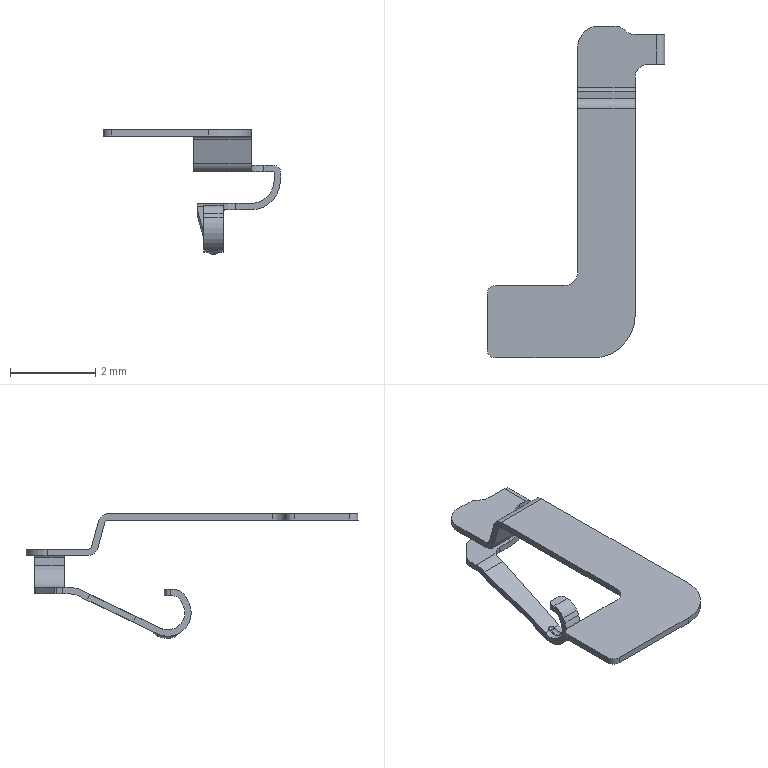Part | STEP file | p9-frame-02 | 1 solid | 70 faces | box 4.174 x 7.792 x 2.928 mm | volume 2.811 mm3 | plane 31 | cylinder 29 | spline 10 | commonest cylinder face diameters 0.4 x5 0.6 x5 1 x4 0.2 x2 0.3 x2 0.5 x2